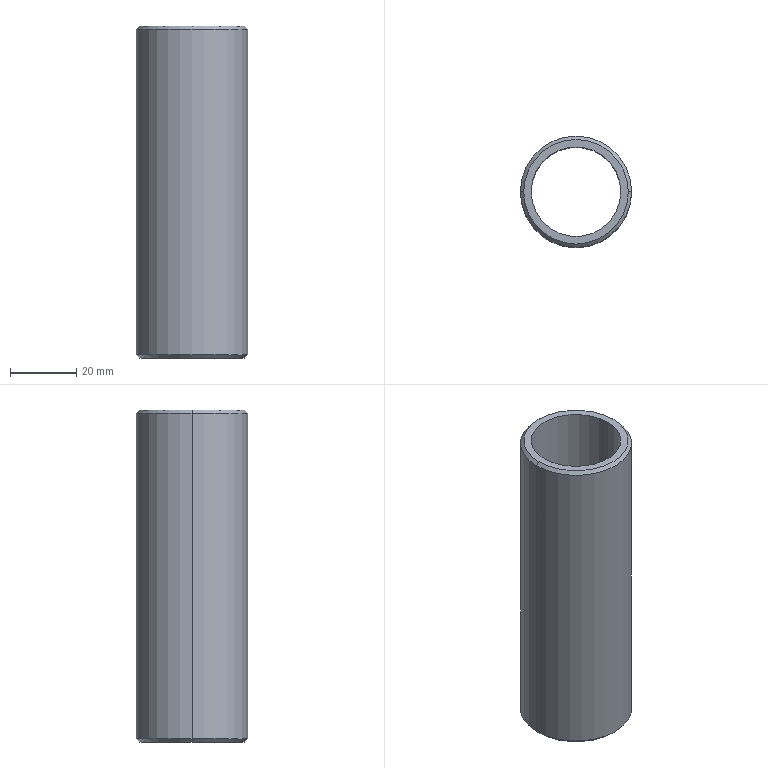Part | SolidWorks | features Chamfer 2, Extrusion 1 | 1 solid | 10 faces | box 33.5 x 33.5 x 100 mm | volume 30783 mm3 | cone 4 | cylinder 4 | plane 2 | commonest cylinder face diameters 27 x2 33.5 x2
STEP:
#1=CARTESIAN_POINT('',(-15.75,0.,0.));
#2=VERTEX_POINT('',#1);
#3=CARTESIAN_POINT('',(15.75,0.,0.));
#4=VERTEX_POINT('',#3);
#5=CARTESIAN_POINT('',(0.,0.,0.));
#6=DIRECTION('',(0.,0.,-1.));
#7=DIRECTION('',(1.,0.,0.));
#8=AXIS2_PLACEMENT_3D('',#5,#6,#7);
#9=CIRCLE('',#8,15.75);
#10=EDGE_CURVE('',#2,#4,#9,.T.);
#11=ORIENTED_EDGE('',*,*,#10,.F.);
#12=CARTESIAN_POINT('',(-16.75,0.,1.));
#13=VERTEX_POINT('',#12);
#14=CARTESIAN_POINT('',(-16.75,0.,1.));
#15=DIRECTION('',(-0.7071,0.,0.7071));
#16=VECTOR('',#15,1000.);
#17=LINE('',#14,#16);
#18=EDGE_CURVE('',#2,#13,#17,.T.);
#19=ORIENTED_EDGE('',*,*,#18,.T.);
#20=CARTESIAN_POINT('',(16.75,0.,1.));
#21=VERTEX_POINT('',#20);
#22=CARTESIAN_POINT('',(0.,0.,1.));
#23=DIRECTION('',(0.,0.,1.));
#24=DIRECTION('',(1.,0.,0.));
#25=AXIS2_PLACEMENT_3D('',#22,#23,#24);
#26=CIRCLE('',#25,16.75);
#27=EDGE_CURVE('',#21,#13,#26,.T.);
#28=ORIENTED_EDGE('',*,*,#27,.F.);
#29=CARTESIAN_POINT('',(16.75,0.,1.));
#30=DIRECTION('',(0.7071,0.,0.7071));
#31=VECTOR('',#30,1000.);
#32=LINE('',#29,#31);
#33=EDGE_CURVE('',#4,#21,#32,.T.);
#34=ORIENTED_EDGE('',*,*,#33,.F.);
#35=EDGE_LOOP('',(#11,#19,#28,#34));
#36=FACE_OUTER_BOUND('',#35,.T.);
#37=CARTESIAN_POINT('',(0.,0.,1.));
#38=DIRECTION('',(0.,0.,1.));
#39=DIRECTION('',(1.,0.,0.));
#40=AXIS2_PLACEMENT_3D('',#37,#38,#39);
#41=CONICAL_SURFACE('',#40,16.75,0.7854);
#42=ADVANCED_FACE('',(#36),#41,.T.);
#43=CARTESIAN_POINT('',(15.75,0.,100.));
#44=VERTEX_POINT('',#43);
#45=CARTESIAN_POINT('',(-15.75,0.,100.));
#46=VERTEX_POINT('',#45);
#47=CARTESIAN_POINT('',(0.,0.,100.));
#48=DIRECTION('',(0.,0.,1.));
#49=DIRECTION('',(1.,0.,0.));
#50=AXIS2_PLACEMENT_3D('',#47,#48,#49);
#51=CIRCLE('',#50,15.75);
#52=EDGE_CURVE('',#44,#46,#51,.T.);
#53=ORIENTED_EDGE('',*,*,#52,.F.);
#54=CARTESIAN_POINT('',(16.75,0.,99.));
#55=VERTEX_POINT('',#54);
#56=CARTESIAN_POINT('',(15.75,0.,100.));
#57=DIRECTION('',(0.7071,0.,-0.7071));
#58=VECTOR('',#57,1000.);
#59=LINE('',#56,#58);
#60=EDGE_CURVE('',#44,#55,#59,.T.);
#61=ORIENTED_EDGE('',*,*,#60,.T.);
#62=CARTESIAN_POINT('',(-16.75,0.,99.));
#63=VERTEX_POINT('',#62);
#64=CARTESIAN_POINT('',(0.,0.,99.));
#65=DIRECTION('',(0.,0.,-1.));
#66=DIRECTION('',(1.,0.,0.));
#67=AXIS2_PLACEMENT_3D('',#64,#65,#66);
#68=CIRCLE('',#67,16.75);
#69=EDGE_CURVE('',#63,#55,#68,.T.);
#70=ORIENTED_EDGE('',*,*,#69,.F.);
#71=CARTESIAN_POINT('',(-15.75,0.,100.));
#72=DIRECTION('',(-0.7071,0.,-0.7071));
#73=VECTOR('',#72,1000.);
#74=LINE('',#71,#73);
#75=EDGE_CURVE('',#46,#63,#74,.T.);
#76=ORIENTED_EDGE('',*,*,#75,.F.);
#77=EDGE_LOOP('',(#53,#61,#70,#76));
#78=FACE_OUTER_BOUND('',#77,.T.);
#79=CARTESIAN_POINT('',(0.,0.,100.));
#80=DIRECTION('',(0.,0.,-1.));
#81=DIRECTION('',(-1.,0.,0.));
#82=AXIS2_PLACEMENT_3D('',#79,#80,#81);
#83=CONICAL_SURFACE('',#82,15.75,0.7854);
#84=ADVANCED_FACE('',(#78),#83,.T.);
#85=CARTESIAN_POINT('',(-13.5,0.,100.));
#86=VERTEX_POINT('',#85);
#87=CARTESIAN_POINT('',(13.5,0.,100.));
#88=VERTEX_POINT('',#87);
#89=CARTESIAN_POINT('',(0.,0.,100.));
#90=DIRECTION('',(0.,0.,1.));
#91=DIRECTION('',(1.,0.,0.));
#92=AXIS2_PLACEMENT_3D('',#89,#90,#91);
#93=CIRCLE('',#92,13.5);
#94=EDGE_CURVE('',#86,#88,#93,.T.);
#95=ORIENTED_EDGE('',*,*,#94,.T.);
#96=CARTESIAN_POINT('',(13.5,0.,0.));
#97=VERTEX_POINT('',#96);
#98=CARTESIAN_POINT('',(13.5,0.,100.));
#99=DIRECTION('',(0.,0.,-1.));
#100=VECTOR('',#99,1000.);
#101=LINE('',#98,#100);
#102=EDGE_CURVE('',#88,#97,#101,.T.);
#103=ORIENTED_EDGE('',*,*,#102,.T.);
#104=CARTESIAN_POINT('',(-13.5,0.,0.));
#105=VERTEX_POINT('',#104);
#106=CARTESIAN_POINT('',(0.,0.,0.));
#107=DIRECTION('',(0.,0.,1.));
#108=DIRECTION('',(1.,0.,0.));
#109=AXIS2_PLACEMENT_3D('',#106,#107,#108);
#110=CIRCLE('',#109,13.5);
#111=EDGE_CURVE('',#105,#97,#110,.T.);
#112=ORIENTED_EDGE('',*,*,#111,.F.);
#113=CARTESIAN_POINT('',(-13.5,0.,100.));
#114=DIRECTION('',(0.,0.,-1.));
#115=VECTOR('',#114,1000.);
#116=LINE('',#113,#115);
#117=EDGE_CURVE('',#86,#105,#116,.T.);
#118=ORIENTED_EDGE('',*,*,#117,.F.);
#119=EDGE_LOOP('',(#95,#103,#112,#118));
#120=FACE_OUTER_BOUND('',#119,.T.);
#121=CARTESIAN_POINT('',(0.,0.,100.));
#122=DIRECTION('',(0.,0.,-1.));
#123=DIRECTION('',(-1.,0.,0.));
#124=AXIS2_PLACEMENT_3D('',#121,#122,#123);
#125=CYLINDRICAL_SURFACE('',#124,13.5);
#126=ADVANCED_FACE('',(#120),#125,.F.);
#127=ORIENTED_EDGE('',*,*,#69,.T.);
#128=CARTESIAN_POINT('',(16.75,0.,100.));
#129=DIRECTION('',(0.,0.,-1.));
#130=VECTOR('',#129,1000.);
#131=LINE('',#128,#130);
#132=EDGE_CURVE('',#55,#21,#131,.T.);
#133=ORIENTED_EDGE('',*,*,#132,.T.);
#134=ORIENTED_EDGE('',*,*,#27,.T.);
#135=CARTESIAN_POINT('',(-16.75,0.,100.));
#136=DIRECTION('',(0.,0.,-1.));
#137=VECTOR('',#136,1000.);
#138=LINE('',#135,#137);
#139=EDGE_CURVE('',#63,#13,#138,.T.);
#140=ORIENTED_EDGE('',*,*,#139,.F.);
#141=EDGE_LOOP('',(#127,#133,#134,#140));
#142=FACE_OUTER_BOUND('',#141,.T.);
#143=CARTESIAN_POINT('',(0.,0.,100.));
#144=DIRECTION('',(0.,0.,-1.));
#145=DIRECTION('',(-1.,0.,0.));
#146=AXIS2_PLACEMENT_3D('',#143,#144,#145);
#147=CYLINDRICAL_SURFACE('',#146,16.75);
#148=ADVANCED_FACE('',(#142),#147,.T.);
#149=CARTESIAN_POINT('',(0.,0.,100.));
#150=DIRECTION('',(0.,0.,1.));
#151=DIRECTION('',(1.,0.,0.));
#152=AXIS2_PLACEMENT_3D('',#149,#150,#151);
#153=CIRCLE('',#152,15.75);
#154=EDGE_CURVE('',#46,#44,#153,.T.);
#155=ORIENTED_EDGE('',*,*,#154,.T.);
#156=ORIENTED_EDGE('',*,*,#52,.T.);
#157=EDGE_LOOP('',(#155,#156));
#158=FACE_OUTER_BOUND('',#157,.T.);
#159=ORIENTED_EDGE('',*,*,#94,.F.);
#160=CARTESIAN_POINT('',(0.,0.,100.));
#161=DIRECTION('',(0.,0.,1.));
#162=DIRECTION('',(1.,0.,0.));
#163=AXIS2_PLACEMENT_3D('',#160,#161,#162);
#164=CIRCLE('',#163,13.5);
#165=EDGE_CURVE('',#88,#86,#164,.T.);
#166=ORIENTED_EDGE('',*,*,#165,.F.);
#167=EDGE_LOOP('',(#159,#166));
#168=FACE_BOUND('',#167,.T.);
#169=CARTESIAN_POINT('',(0.,0.,100.));
#170=DIRECTION('',(0.,0.,1.));
#171=DIRECTION('',(1.,0.,0.));
#172=AXIS2_PLACEMENT_3D('',#169,#170,#171);
#173=PLANE('',#172);
#174=ADVANCED_FACE('',(#158,#168),#173,.T.);
#175=CARTESIAN_POINT('',(0.,0.,0.));
#176=DIRECTION('',(0.,0.,-1.));
#177=DIRECTION('',(1.,0.,0.));
#178=AXIS2_PLACEMENT_3D('',#175,#176,#177);
#179=CIRCLE('',#178,15.75);
#180=EDGE_CURVE('',#4,#2,#179,.T.);
#181=ORIENTED_EDGE('',*,*,#180,.T.);
#182=ORIENTED_EDGE('',*,*,#10,.T.);
#183=EDGE_LOOP('',(#181,#182));
#184=FACE_OUTER_BOUND('',#183,.T.);
#185=ORIENTED_EDGE('',*,*,#111,.T.);
#186=CARTESIAN_POINT('',(0.,0.,0.));
#187=DIRECTION('',(0.,0.,1.));
#188=DIRECTION('',(1.,0.,0.));
#189=AXIS2_PLACEMENT_3D('',#186,#187,#188);
#190=CIRCLE('',#189,13.5);
#191=EDGE_CURVE('',#97,#105,#190,.T.);
#192=ORIENTED_EDGE('',*,*,#191,.T.);
#193=EDGE_LOOP('',(#185,#192));
#194=FACE_BOUND('',#193,.T.);
#195=CARTESIAN_POINT('',(0.,0.,0.));
#196=DIRECTION('',(0.,0.,1.));
#197=DIRECTION('',(1.,0.,0.));
#198=AXIS2_PLACEMENT_3D('',#195,#196,#197);
#199=PLANE('',#198);
#200=ADVANCED_FACE('',(#184,#194),#199,.F.);
#201=ORIENTED_EDGE('',*,*,#132,.F.);
#202=CARTESIAN_POINT('',(0.,0.,99.));
#203=DIRECTION('',(0.,0.,-1.));
#204=DIRECTION('',(1.,0.,0.));
#205=AXIS2_PLACEMENT_3D('',#202,#203,#204);
#206=CIRCLE('',#205,16.75);
#207=EDGE_CURVE('',#55,#63,#206,.T.);
#208=ORIENTED_EDGE('',*,*,#207,.T.);
#209=ORIENTED_EDGE('',*,*,#139,.T.);
#210=CARTESIAN_POINT('',(0.,0.,1.));
#211=DIRECTION('',(0.,0.,1.));
#212=DIRECTION('',(1.,0.,0.));
#213=AXIS2_PLACEMENT_3D('',#210,#211,#212);
#214=CIRCLE('',#213,16.75);
#215=EDGE_CURVE('',#13,#21,#214,.T.);
#216=ORIENTED_EDGE('',*,*,#215,.T.);
#217=EDGE_LOOP('',(#201,#208,#209,#216));
#218=FACE_OUTER_BOUND('',#217,.T.);
#219=CARTESIAN_POINT('',(0.,0.,100.));
#220=DIRECTION('',(0.,0.,-1.));
#221=DIRECTION('',(-1.,0.,0.));
#222=AXIS2_PLACEMENT_3D('',#219,#220,#221);
#223=CYLINDRICAL_SURFACE('',#222,16.75);
#224=ADVANCED_FACE('',(#218),#223,.T.);
#225=ORIENTED_EDGE('',*,*,#102,.F.);
#226=ORIENTED_EDGE('',*,*,#165,.T.);
#227=ORIENTED_EDGE('',*,*,#117,.T.);
#228=ORIENTED_EDGE('',*,*,#191,.F.);
#229=EDGE_LOOP('',(#225,#226,#227,#228));
#230=FACE_OUTER_BOUND('',#229,.T.);
#231=CARTESIAN_POINT('',(0.,0.,100.));
#232=DIRECTION('',(0.,0.,-1.));
#233=DIRECTION('',(-1.,0.,0.));
#234=AXIS2_PLACEMENT_3D('',#231,#232,#233);
#235=CYLINDRICAL_SURFACE('',#234,13.5);
#236=ADVANCED_FACE('',(#230),#235,.F.);
#237=ORIENTED_EDGE('',*,*,#60,.F.);
#238=ORIENTED_EDGE('',*,*,#154,.F.);
#239=ORIENTED_EDGE('',*,*,#75,.T.);
#240=ORIENTED_EDGE('',*,*,#207,.F.);
#241=EDGE_LOOP('',(#237,#238,#239,#240));
#242=FACE_OUTER_BOUND('',#241,.T.);
#243=CARTESIAN_POINT('',(0.,0.,100.));
#244=DIRECTION('',(0.,0.,-1.));
#245=DIRECTION('',(-1.,0.,0.));
#246=AXIS2_PLACEMENT_3D('',#243,#244,#245);
#247=CONICAL_SURFACE('',#246,15.75,0.7854);
#248=ADVANCED_FACE('',(#242),#247,.T.);
#249=ORIENTED_EDGE('',*,*,#18,.F.);
#250=ORIENTED_EDGE('',*,*,#180,.F.);
#251=ORIENTED_EDGE('',*,*,#33,.T.);
#252=ORIENTED_EDGE('',*,*,#215,.F.);
#253=EDGE_LOOP('',(#249,#250,#251,#252));
#254=FACE_OUTER_BOUND('',#253,.T.);
#255=CARTESIAN_POINT('',(0.,0.,1.));
#256=DIRECTION('',(0.,0.,1.));
#257=DIRECTION('',(1.,0.,0.));
#258=AXIS2_PLACEMENT_3D('',#255,#256,#257);
#259=CONICAL_SURFACE('',#258,16.75,0.7854);
#260=ADVANCED_FACE('',(#254),#259,.T.);
#261=CLOSED_SHELL('',(#42,#84,#126,#148,#174,#200,#224,#236,#248,#260));
#262=MANIFOLD_SOLID_BREP('',#261);
#263=CARTESIAN_POINT('',(0.,0.,0.));
#264=DIRECTION('',(0.,0.,1.));
#265=DIRECTION('',(1.,0.,0.));
#266=AXIS2_PLACEMENT_3D('',#263,#264,#265);
#267=(LENGTH_UNIT()NAMED_UNIT(*)SI_UNIT(.MILLI.,.METRE.));
#268=UNCERTAINTY_MEASURE_WITH_UNIT(LENGTH_MEASURE(0.00001),#267,'','');
#269=(NAMED_UNIT(*)PLANE_ANGLE_UNIT()SI_UNIT($,.RADIAN.));
#270=(NAMED_UNIT(*)SI_UNIT($,.STERADIAN.)SOLID_ANGLE_UNIT());
#271=(GEOMETRIC_REPRESENTATION_CONTEXT(3)GLOBAL_UNCERTAINTY_ASSIGNED_CONTEXT((#268))GLOBAL_UNIT_ASSIGNED_CONTEXT((#267,#269,#270))REPRESENTATION_CONTEXT('',''));
#272=ADVANCED_BREP_SHAPE_REPRESENTATION('',(#262,#266),#271);